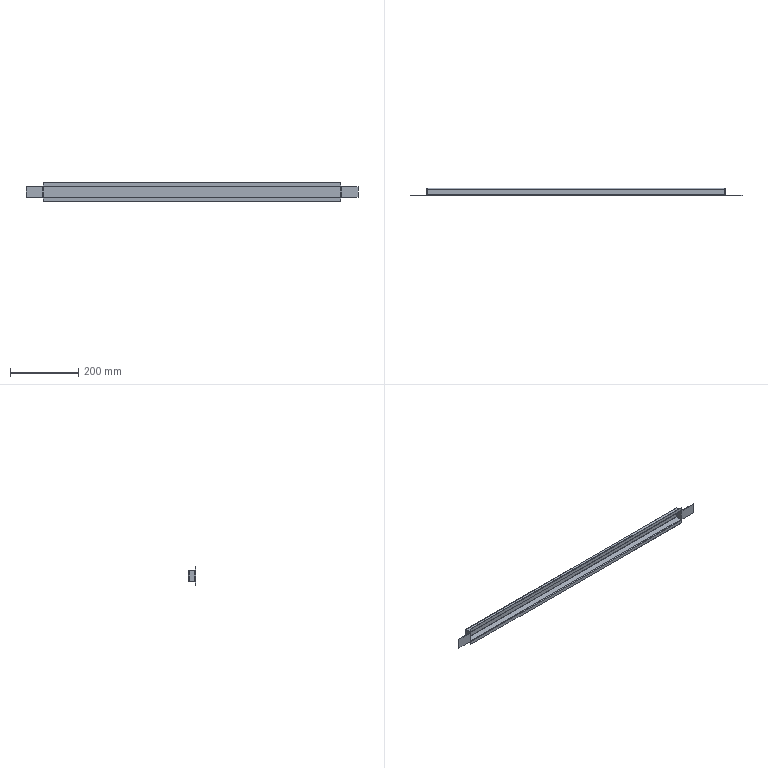Part | STEP file | 750078362 | 1 solid | 54 faces | box 974 x 21.5 x 55 mm | volume 128141 mm3 | plane 38 | cylinder 16 | commonest cylinder face diameters 1 x8 4 x8